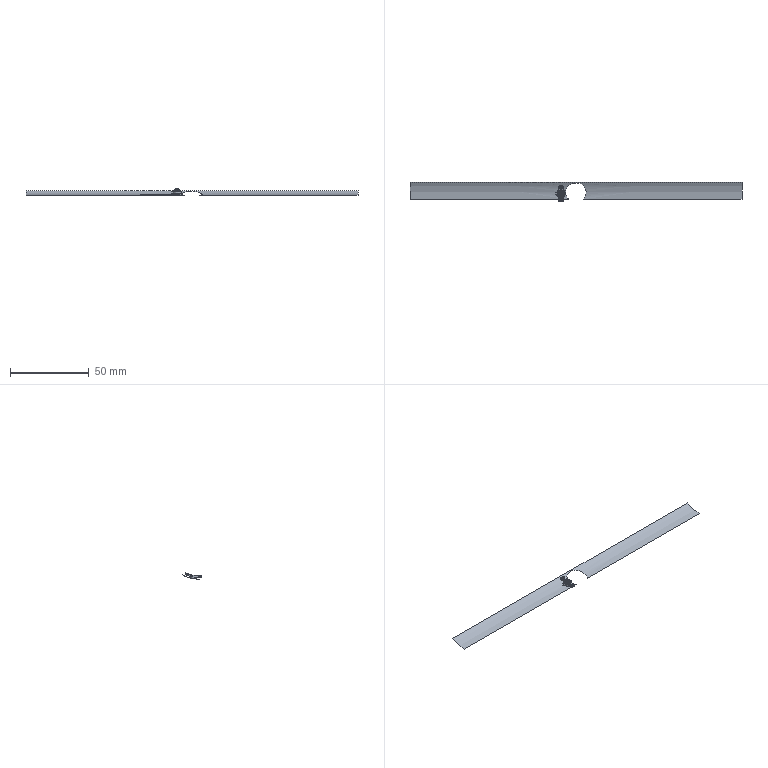Part | Creo | 1 solid | 74 faces | box 211.4 x 12.505 x 3.981 mm | volume 1559 mm3 | cone 34 | cylinder 21 | plane 9 | other 6 | spline 4 | commonest cylinder face diameters 2 x8 1 x4 5.5 x3 3.5 x2 4.1 x2 4.4 x1